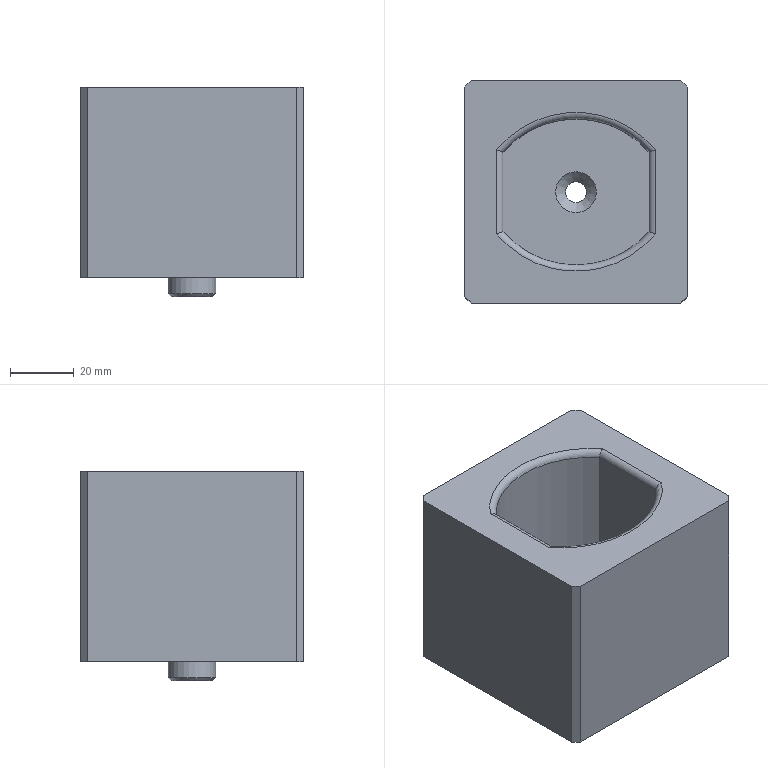NC program | NX | posted with a generic post | part box 70 x 70 x 66 mm
Lines 6219 to 6380 of 8582:
(ZLEVEL_PROFILE_COPY_COPY , TOOL : D10)
N12424 T04 M6
N12426 G54
N12428 G17 G0 G90 X-15.383 Y10.246 S7500 M3
N12430 G43 Z30. H4
N12432 Z-7.642
N12434 G94 G1 Z-9.142 F1000.
N12436 X-17.024 Y10.758
N12438 G3 X-17.999 Y10.538 R1.
N12440 G1 X-18. Y10.537 F850.
N12442 Y-10.349
N12444 X-18.004 Y-10.534
N12446 G3 X18. Y-10.538 R25.44
N12448 G1 Y10.538
N12450 G3 X-17.999 Y10.538 R25.44
N12452 X-17.499 Y9.672 R1.
N12454 G1 X-16. Y8.807
N12456 Z-7.642
N12458 G0 X-15.383 Y10.246 Z-16.783
N12460 G1 Z-18.283 F1000.
N12462 X-17.024 Y10.758
N12464 G3 X-17.999 Y10.538 R1.
N12466 G1 X-18. Y10.537 F850.
N12468 Y-10.349
N12470 X-18.003 Y-10.534
N12472 G3 X18. Y-10.538 R25.44
N12474 G1 Y10.537
N12476 X17.908 Y10.63
N12478 G3 X-17.999 Y10.538 R25.44
N12480 X-17.499 Y9.672 R1.
N12482 G1 X-16. Y8.807
N12484 Z-16.783
N12486 G0 X-15.383 Y10.246 Z-25.925
N12488 G1 Z-27.425 F1000.
N12490 X-17.024 Y10.758
N12492 G3 X-17.999 Y10.538 R1.
N12494 G1 X-18. Y10.536 F850.
N12496 Y-10.349
N12498 X-18.002 Y-10.535
N12500 G3 X18. Y-10.538 R25.44
N12502 G1 Y10.536
N12504 X17.907 Y10.63
N12506 G3 X-17.999 Y10.538 R25.44
N12508 X-17.499 Y9.672 R1.
N12510 G1 X-16. Y8.807
N12512 Z-25.925
N12514 G0 X-15.383 Y10.246 Z-35.067
N12516 G1 Z-36.567 F1000.
N12518 X-17.023 Y10.758
N12520 G3 X-17.999 Y10.538 R1.
N12522 G1 X-18. Y10.536 F850.
N12524 Y-10.349
N12526 X-18.002 Y-10.536
N12528 G3 X18. Y-10.538 R25.44
N12530 G1 Y10.536
N12532 X17.907 Y10.63
N12534 G3 X-17.999 Y10.538 R25.44
N12536 X-17.499 Y9.672 R1.
N12538 G1 X-16. Y8.807
N12540 Z-35.067
N12542 G0 X-15.383 Y10.246 Z-44.208
N12544 G1 Z-45.708 F1000.
N12546 X-17.023 Y10.758
N12548 G3 X-17.999 Y10.538 R1.
N12550 G1 X-18. Y10.536 F850.
N12552 Y-10.349
N12554 X-18.001 Y-10.537
N12556 G3 X18. Y-10.538 R25.44
N12558 G1 Y10.536
N12560 X17.907 Y10.631
N12562 G3 X-17.999 Y10.538 R25.44
N12564 X-17.499 Y9.672 R1.
N12566 G1 X-16. Y8.807
N12568 Z-44.208
N12570 G0 X-15.383 Y10.246 Z-53.35
N12572 G1 Z-54.85 F1000.
N12574 X-17.023 Y10.757
N12576 G3 X-17.999 Y10.538 R1.
N12578 G1 X-18. Y10.535 F850.
N12580 Y-10.538
N12582 G3 X18. Y-10.538 R25.44
N12584 G1 Y10.535
N12586 X17.907 Y10.631
N12588 G3 X-17.999 Y10.538 R25.44
N12590 X-17.499 Y9.672 R1.
N12592 G1 X-16. Y8.807
N12594 Z-53.35
N12596 G0 Z30.
(FLOOR_WALL_1_COPY_COPY , TOOL : D10)
N12598 X-16.997 Y-9.467
N12600 Z-53.5
N12602 G1 Z-55. F1000.
N12604 G3 X-17.497 Y-10.333 R1.
N12606 G1 Y10.333
N12608 G2 X-10.498 Y15.183 R24.94
N12610 G1 Y-15.183
N12612 G3 X-3.498 Y-17.253 R24.94
N12614 G1 Y17.253
N12616 G2 X3.501 Y17.253 R24.94
N12618 G1 Y-17.253
N12620 G3 X10.501 Y-15.182 R24.94
N12622 G1 Y15.182
N12624 G2 X17.5 Y10.33 R24.94
N12626 G1 Y-10.33
N12628 X16.883 Y-10.937
N12630 G3 X17.851 Y-10.686 R1.
N12632 X18. Y-10.538 R25.44
N12634 G1 Y10.538
N12636 G3 X-18. Y10.538 R25.44
N12638 G1 Y-10.538
N12640 G3 X17.851 Y-10.686 R25.44
N12642 X17.984 Y-10.204 R0.5
N12644 G1 X16.5 Y-4.491
N12646 Z-53.5
N12648 G0 Z30.
N12650 M5
(PLANAR_MILL_COPY_COPY , TOOL : D8A45)
N12652 T06 M6
N12654 G54
N12656 G17 G0 G90 X-40.3 Y0. S7500 M3
N12658 G43 Z30. H6
N12660 Z1.5
N12662 G94 G1 Z-1.5 F1250.
N12664 X-36.3
N12666 Y33.
N12668 G2 X-35.919 Y33.919 R1.3
N12670 G1 X-33.919 Y35.919
N12672 G2 X-33. Y36.3 R1.3
N12674 G1 X33.
N12676 G2 X33.919 Y35.919 R1.3
N12678 G1 X35.919 Y33.919
N12680 G2 X36.3 Y33. R1.3
N12682 G1 Y-33.
N12684 G2 X35.919 Y-33.919 R1.3
N12686 G1 X33.919 Y-35.919
N12688 G2 X33. Y-36.3 R1.3
N12690 G1 X-33.
N12692 G2 X-33.919 Y-35.919 R1.3
N12694 G1 X-35.919 Y-33.919
N12696 G2 X-36.3 Y-33. R1.3
N12698 G1 Y0.
N12700 X-40.3
N12702 Z1.5
N12704 G0 Z30.
N12706 M5
(DRILLING_COPY_1 , TOOL : 14.0ZT)
N12708 T18 M6
N12710 G54
N12712 G17 G0 G90 X0. Y0. S3000 M3
N12714 G43 Z30. H18
N12716 G94 G81 G98 Z-61.4 F250. R-52.
N12718 G80
N12720 G0 X0. Y0. Z30.
N12722 M5